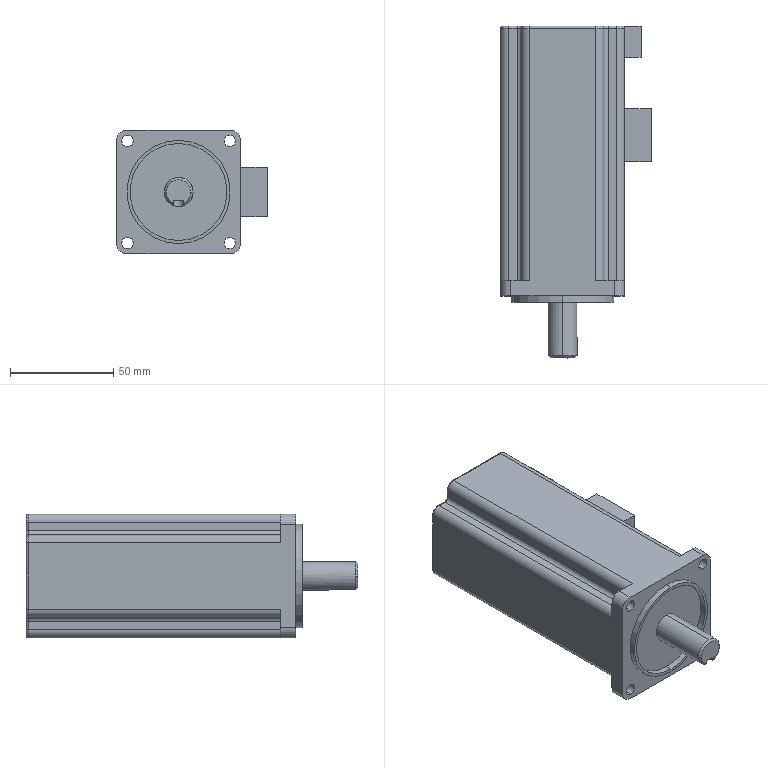Part | STEP file | TD400W | 1 solid | 93 faces | box 73 x 160.7 x 60 mm | volume 432844 mm3 | cylinder 43 | plane 35 | spline 12 | cone 3 | commonest cylinder face diameters 2 x12 5.5 x8 8 x8 4 x4 10 x4 14 x2